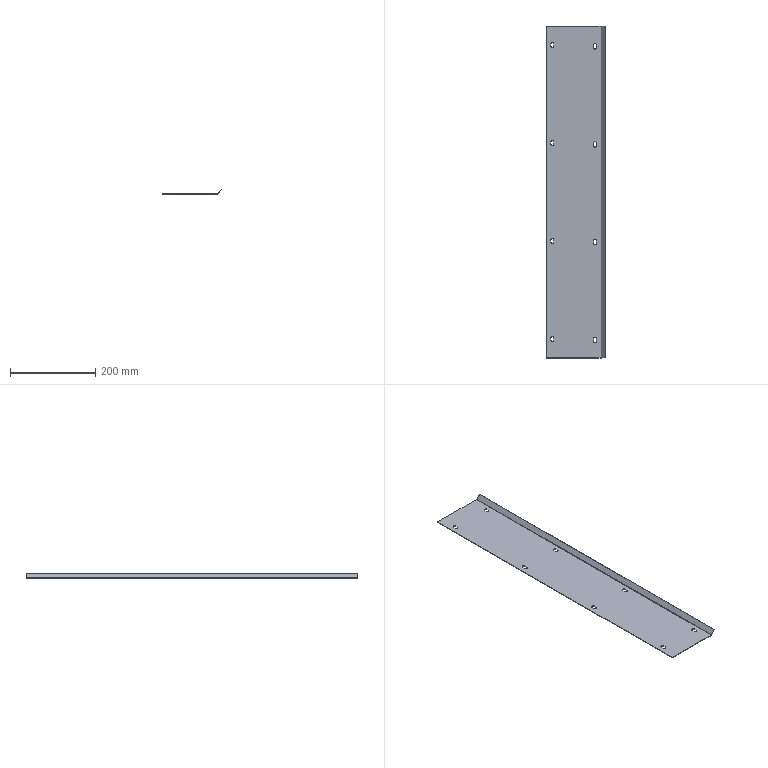Part | SolidWorks | features ICE 2, EdgeFlange 1, FlatPattern 1, LPattern 1, SMBaseFlange 1, SheetMetal 1 | 1 solid | 46 faces | box 140.607 x 780 x 11.455 mm | volume 134418 mm3 | plane 28 | cylinder 18 | commonest cylinder face diameters 7 x16 2 x1 4.4 x1
STEP:
#1=CARTESIAN_POINT('',(46.455,-345.,-1.2));
#2=VERTEX_POINT('',#1);
#3=CARTESIAN_POINT('',(46.455,-345.,0.));
#4=VERTEX_POINT('',#3);
#5=CARTESIAN_POINT('',(46.455,-345.,-10.));
#6=DIRECTION('',(0.,0.,1.));
#7=VECTOR('',#6,1000.);
#8=LINE('',#5,#7);
#9=EDGE_CURVE('',#2,#4,#8,.T.);
#10=ORIENTED_EDGE('',*,*,#9,.T.);
#11=CARTESIAN_POINT('',(46.455,-351.,0.));
#12=VERTEX_POINT('',#11);
#13=CARTESIAN_POINT('',(46.455,-345.,0.));
#14=DIRECTION('',(0.,-1.,0.));
#15=VECTOR('',#14,1000.);
#16=LINE('',#13,#15);
#17=EDGE_CURVE('',#4,#12,#16,.T.);
#18=ORIENTED_EDGE('',*,*,#17,.T.);
#19=CARTESIAN_POINT('',(46.455,-351.,-1.2));
#20=VERTEX_POINT('',#19);
#21=CARTESIAN_POINT('',(46.455,-351.,-10.));
#22=DIRECTION('',(0.,0.,1.));
#23=VECTOR('',#22,1000.);
#24=LINE('',#21,#23);
#25=EDGE_CURVE('',#20,#12,#24,.T.);
#26=ORIENTED_EDGE('',*,*,#25,.F.);
#27=CARTESIAN_POINT('',(46.455,-690.,-1.2));
#28=DIRECTION('',(0.,-1.,0.));
#29=VECTOR('',#28,1000.);
#30=LINE('',#27,#29);
#31=EDGE_CURVE('',#2,#20,#30,.T.);
#32=ORIENTED_EDGE('',*,*,#31,.F.);
#33=EDGE_LOOP('',(#10,#18,#26,#32));
#34=FACE_OUTER_BOUND('',#33,.T.);
#35=CARTESIAN_POINT('',(46.455,-345.,-10.));
#36=DIRECTION('',(-1.,0.,0.));
#37=DIRECTION('',(0.,0.,1.));
#38=AXIS2_PLACEMENT_3D('',#35,#36,#37);
#39=PLANE('',#38);
#40=ADVANCED_FACE('',(#34),#39,.F.);
#41=ORIENTED_EDGE('',*,*,#25,.T.);
#42=CARTESIAN_POINT('',(53.455,-351.,0.));
#43=VERTEX_POINT('',#42);
#44=CARTESIAN_POINT('',(49.955,-351.,0.));
#45=DIRECTION('',(0.,0.,1.));
#46=DIRECTION('',(1.,0.,0.));
#47=AXIS2_PLACEMENT_3D('',#44,#45,#46);
#48=CIRCLE('',#47,3.5);
#49=EDGE_CURVE('',#12,#43,#48,.T.);
#50=ORIENTED_EDGE('',*,*,#49,.T.);
#51=CARTESIAN_POINT('',(53.455,-351.,-1.2));
#52=VERTEX_POINT('',#51);
#53=CARTESIAN_POINT('',(53.455,-351.,-10.));
#54=DIRECTION('',(0.,0.,1.));
#55=VECTOR('',#54,1000.);
#56=LINE('',#53,#55);
#57=EDGE_CURVE('',#52,#43,#56,.T.);
#58=ORIENTED_EDGE('',*,*,#57,.F.);
#59=CARTESIAN_POINT('',(49.955,-351.,-1.2));
#60=DIRECTION('',(0.,0.,1.));
#61=DIRECTION('',(1.,0.,0.));
#62=AXIS2_PLACEMENT_3D('',#59,#60,#61);
#63=CIRCLE('',#62,3.5);
#64=EDGE_CURVE('',#20,#52,#63,.T.);
#65=ORIENTED_EDGE('',*,*,#64,.F.);
#66=EDGE_LOOP('',(#41,#50,#58,#65));
#67=FACE_OUTER_BOUND('',#66,.T.);
#68=CARTESIAN_POINT('',(49.955,-351.,-10.));
#69=DIRECTION('',(0.,0.,1.));
#70=DIRECTION('',(1.,0.,0.));
#71=AXIS2_PLACEMENT_3D('',#68,#69,#70);
#72=CYLINDRICAL_SURFACE('',#71,3.5);
#73=ADVANCED_FACE('',(#67),#72,.F.);
#74=ORIENTED_EDGE('',*,*,#57,.T.);
#75=CARTESIAN_POINT('',(53.455,-345.,0.));
#76=VERTEX_POINT('',#75);
#77=CARTESIAN_POINT('',(53.455,-345.,0.));
#78=DIRECTION('',(0.,1.,0.));
#79=VECTOR('',#78,1000.);
#80=LINE('',#77,#79);
#81=EDGE_CURVE('',#43,#76,#80,.T.);
#82=ORIENTED_EDGE('',*,*,#81,.T.);
#83=CARTESIAN_POINT('',(53.455,-345.,-1.2));
#84=VERTEX_POINT('',#83);
#85=CARTESIAN_POINT('',(53.455,-345.,-10.));
#86=DIRECTION('',(0.,0.,1.));
#87=VECTOR('',#86,1000.);
#88=LINE('',#85,#87);
#89=EDGE_CURVE('',#84,#76,#88,.T.);
#90=ORIENTED_EDGE('',*,*,#89,.F.);
#91=CARTESIAN_POINT('',(53.455,-690.,-1.2));
#92=DIRECTION('',(0.,1.,0.));
#93=VECTOR('',#92,1000.);
#94=LINE('',#91,#93);
#95=EDGE_CURVE('',#52,#84,#94,.T.);
#96=ORIENTED_EDGE('',*,*,#95,.F.);
#97=EDGE_LOOP('',(#74,#82,#90,#96));
#98=FACE_OUTER_BOUND('',#97,.T.);
#99=CARTESIAN_POINT('',(53.455,-345.,-10.));
#100=DIRECTION('',(1.,0.,0.));
#101=DIRECTION('',(0.,0.,-1.));
#102=AXIS2_PLACEMENT_3D('',#99,#100,#101);
#103=PLANE('',#102);
#104=ADVANCED_FACE('',(#98),#103,.F.);
#105=ORIENTED_EDGE('',*,*,#89,.T.);
#106=CARTESIAN_POINT('',(49.955,-345.,0.));
#107=DIRECTION('',(0.,0.,1.));
#108=DIRECTION('',(1.,0.,0.));
#109=AXIS2_PLACEMENT_3D('',#106,#107,#108);
#110=CIRCLE('',#109,3.5);
#111=EDGE_CURVE('',#76,#4,#110,.T.);
#112=ORIENTED_EDGE('',*,*,#111,.T.);
#113=ORIENTED_EDGE('',*,*,#9,.F.);
#114=CARTESIAN_POINT('',(49.955,-345.,-1.2));
#115=DIRECTION('',(0.,0.,1.));
#116=DIRECTION('',(1.,0.,0.));
#117=AXIS2_PLACEMENT_3D('',#114,#115,#116);
#118=CIRCLE('',#117,3.5);
#119=EDGE_CURVE('',#84,#2,#118,.T.);
#120=ORIENTED_EDGE('',*,*,#119,.F.);
#121=EDGE_LOOP('',(#105,#112,#113,#120));
#122=FACE_OUTER_BOUND('',#121,.T.);
#123=CARTESIAN_POINT('',(49.955,-345.,-10.));
#124=DIRECTION('',(0.,0.,1.));
#125=DIRECTION('',(1.,0.,0.));
#126=AXIS2_PLACEMENT_3D('',#123,#124,#125);
#127=CYLINDRICAL_SURFACE('',#126,3.5);
#128=ADVANCED_FACE('',(#122),#127,.F.);
#129=CARTESIAN_POINT('',(46.455,-115.,-1.2));
#130=VERTEX_POINT('',#129);
#131=CARTESIAN_POINT('',(46.455,-115.,0.));
#132=VERTEX_POINT('',#131);
#133=CARTESIAN_POINT('',(46.455,-115.,-10.));
#134=DIRECTION('',(0.,0.,1.));
#135=VECTOR('',#134,1000.);
#136=LINE('',#133,#135);
#137=EDGE_CURVE('',#130,#132,#136,.T.);
#138=ORIENTED_EDGE('',*,*,#137,.T.);
#139=CARTESIAN_POINT('',(46.455,-121.,0.));
#140=VERTEX_POINT('',#139);
#141=CARTESIAN_POINT('',(46.455,-115.,0.));
#142=DIRECTION('',(0.,-1.,0.));
#143=VECTOR('',#142,1000.);
#144=LINE('',#141,#143);
#145=EDGE_CURVE('',#132,#140,#144,.T.);
#146=ORIENTED_EDGE('',*,*,#145,.T.);
#147=CARTESIAN_POINT('',(46.455,-121.,-1.2));
#148=VERTEX_POINT('',#147);
#149=CARTESIAN_POINT('',(46.455,-121.,-10.));
#150=DIRECTION('',(0.,0.,1.));
#151=VECTOR('',#150,1000.);
#152=LINE('',#149,#151);
#153=EDGE_CURVE('',#148,#140,#152,.T.);
#154=ORIENTED_EDGE('',*,*,#153,.F.);
#155=CARTESIAN_POINT('',(46.455,-460.,-1.2));
#156=DIRECTION('',(0.,-1.,0.));
#157=VECTOR('',#156,1000.);
#158=LINE('',#155,#157);
#159=EDGE_CURVE('',#130,#148,#158,.T.);
#160=ORIENTED_EDGE('',*,*,#159,.F.);
#161=EDGE_LOOP('',(#138,#146,#154,#160));
#162=FACE_OUTER_BOUND('',#161,.T.);
#163=CARTESIAN_POINT('',(46.455,-115.,-10.));
#164=DIRECTION('',(-1.,0.,0.));
#165=DIRECTION('',(0.,0.,1.));
#166=AXIS2_PLACEMENT_3D('',#163,#164,#165);
#167=PLANE('',#166);
#168=ADVANCED_FACE('',(#162),#167,.F.);
#169=ORIENTED_EDGE('',*,*,#153,.T.);
#170=CARTESIAN_POINT('',(53.455,-121.,0.));
#171=VERTEX_POINT('',#170);
#172=CARTESIAN_POINT('',(49.955,-121.,0.));
#173=DIRECTION('',(0.,0.,1.));
#174=DIRECTION('',(1.,0.,0.));
#175=AXIS2_PLACEMENT_3D('',#172,#173,#174);
#176=CIRCLE('',#175,3.5);
#177=EDGE_CURVE('',#140,#171,#176,.T.);
#178=ORIENTED_EDGE('',*,*,#177,.T.);
#179=CARTESIAN_POINT('',(53.455,-121.,-1.2));
#180=VERTEX_POINT('',#179);
#181=CARTESIAN_POINT('',(53.455,-121.,-10.));
#182=DIRECTION('',(0.,0.,1.));
#183=VECTOR('',#182,1000.);
#184=LINE('',#181,#183);
#185=EDGE_CURVE('',#180,#171,#184,.T.);
#186=ORIENTED_EDGE('',*,*,#185,.F.);
#187=CARTESIAN_POINT('',(49.955,-121.,-1.2));
#188=DIRECTION('',(0.,0.,1.));
#189=DIRECTION('',(1.,0.,0.));
#190=AXIS2_PLACEMENT_3D('',#187,#188,#189);
#191=CIRCLE('',#190,3.5);
#192=EDGE_CURVE('',#148,#180,#191,.T.);
#193=ORIENTED_EDGE('',*,*,#192,.F.);
#194=EDGE_LOOP('',(#169,#178,#186,#193));
#195=FACE_OUTER_BOUND('',#194,.T.);
#196=CARTESIAN_POINT('',(49.955,-121.,-10.));
#197=DIRECTION('',(0.,0.,1.));
#198=DIRECTION('',(1.,0.,0.));
#199=AXIS2_PLACEMENT_3D('',#196,#197,#198);
#200=CYLINDRICAL_SURFACE('',#199,3.5);
#201=ADVANCED_FACE('',(#195),#200,.F.);
#202=ORIENTED_EDGE('',*,*,#185,.T.);
#203=CARTESIAN_POINT('',(53.455,-115.,0.));
#204=VERTEX_POINT('',#203);
#205=CARTESIAN_POINT('',(53.455,-115.,0.));
#206=DIRECTION('',(0.,1.,0.));
#207=VECTOR('',#206,1000.);
#208=LINE('',#205,#207);
#209=EDGE_CURVE('',#171,#204,#208,.T.);
#210=ORIENTED_EDGE('',*,*,#209,.T.);
#211=CARTESIAN_POINT('',(53.455,-115.,-1.2));
#212=VERTEX_POINT('',#211);
#213=CARTESIAN_POINT('',(53.455,-115.,-10.));
#214=DIRECTION('',(0.,0.,1.));
#215=VECTOR('',#214,1000.);
#216=LINE('',#213,#215);
#217=EDGE_CURVE('',#212,#204,#216,.T.);
#218=ORIENTED_EDGE('',*,*,#217,.F.);
#219=CARTESIAN_POINT('',(53.455,-460.,-1.2));
#220=DIRECTION('',(0.,1.,0.));
#221=VECTOR('',#220,1000.);
#222=LINE('',#219,#221);
#223=EDGE_CURVE('',#180,#212,#222,.T.);
#224=ORIENTED_EDGE('',*,*,#223,.F.);
#225=EDGE_LOOP('',(#202,#210,#218,#224));
#226=FACE_OUTER_BOUND('',#225,.T.);
#227=CARTESIAN_POINT('',(53.455,-115.,-10.));
#228=DIRECTION('',(1.,0.,0.));
#229=DIRECTION('',(0.,0.,-1.));
#230=AXIS2_PLACEMENT_3D('',#227,#228,#229);
#231=PLANE('',#230);
#232=ADVANCED_FACE('',(#226),#231,.F.);
#233=ORIENTED_EDGE('',*,*,#217,.T.);
#234=CARTESIAN_POINT('',(49.955,-115.,0.));
#235=DIRECTION('',(0.,0.,1.));
#236=DIRECTION('',(1.,0.,0.));
#237=AXIS2_PLACEMENT_3D('',#234,#235,#236);
#238=CIRCLE('',#237,3.5);
#239=EDGE_CURVE('',#204,#132,#238,.T.);
#240=ORIENTED_EDGE('',*,*,#239,.T.);
#241=ORIENTED_EDGE('',*,*,#137,.F.);
#242=CARTESIAN_POINT('',(49.955,-115.,-1.2));
#243=DIRECTION('',(0.,0.,1.));
#244=DIRECTION('',(1.,0.,0.));
#245=AXIS2_PLACEMENT_3D('',#242,#243,#244);
#246=CIRCLE('',#245,3.5);
#247=EDGE_CURVE('',#212,#130,#246,.T.);
#248=ORIENTED_EDGE('',*,*,#247,.F.);
#249=EDGE_LOOP('',(#233,#240,#241,#248));
#250=FACE_OUTER_BOUND('',#249,.T.);
#251=CARTESIAN_POINT('',(49.955,-115.,-10.));
#252=DIRECTION('',(0.,0.,1.));
#253=DIRECTION('',(1.,0.,0.));
#254=AXIS2_PLACEMENT_3D('',#251,#252,#253);
#255=CYLINDRICAL_SURFACE('',#254,3.5);
#256=ADVANCED_FACE('',(#250),#255,.F.);
#257=CARTESIAN_POINT('',(-53.5,-342.,-1.2));
#258=VERTEX_POINT('',#257);
#259=CARTESIAN_POINT('',(-53.5,-342.,0.));
#260=VERTEX_POINT('',#259);
#261=CARTESIAN_POINT('',(-53.5,-342.,-10.));
#262=DIRECTION('',(0.,0.,1.));
#263=VECTOR('',#262,1000.);
#264=LINE('',#261,#263);
#265=EDGE_CURVE('',#258,#260,#264,.T.);
#266=ORIENTED_EDGE('',*,*,#265,.T.);
#267=CARTESIAN_POINT('',(-53.5,-348.,0.));
#268=VERTEX_POINT('',#267);
#269=CARTESIAN_POINT('',(-53.5,-342.,0.));
#270=DIRECTION('',(0.,-1.,0.));
#271=VECTOR('',#270,1000.);
#272=LINE('',#269,#271);
#273=EDGE_CURVE('',#260,#268,#272,.T.);
#274=ORIENTED_EDGE('',*,*,#273,.T.);
#275=CARTESIAN_POINT('',(-53.5,-348.,-1.2));
#276=VERTEX_POINT('',#275);
#277=CARTESIAN_POINT('',(-53.5,-348.,-10.));
#278=DIRECTION('',(0.,0.,1.));
#279=VECTOR('',#278,1000.);
#280=LINE('',#277,#279);
#281=EDGE_CURVE('',#276,#268,#280,.T.);
#282=ORIENTED_EDGE('',*,*,#281,.F.);
#283=CARTESIAN_POINT('',(-53.5,-690.,-1.2));
#284=DIRECTION('',(0.,-1.,0.));
#285=VECTOR('',#284,1000.);
#286=LINE('',#283,#285);
#287=EDGE_CURVE('',#258,#276,#286,.T.);
#288=ORIENTED_EDGE('',*,*,#287,.F.);
#289=EDGE_LOOP('',(#266,#274,#282,#288));
#290=FACE_OUTER_BOUND('',#289,.T.);
#291=CARTESIAN_POINT('',(-53.5,-342.,-10.));
#292=DIRECTION('',(-1.,0.,0.));
#293=DIRECTION('',(0.,-1.,0.));
#294=AXIS2_PLACEMENT_3D('',#291,#292,#293);
#295=PLANE('',#294);
#296=ADVANCED_FACE('',(#290),#295,.F.);
#297=ORIENTED_EDGE('',*,*,#281,.T.);
#298=CARTESIAN_POINT('',(-46.5,-348.,0.));
#299=VERTEX_POINT('',#298);
#300=CARTESIAN_POINT('',(-50.,-348.,0.));
#301=DIRECTION('',(0.,0.,1.));
#302=DIRECTION('',(1.,0.,0.));
#303=AXIS2_PLACEMENT_3D('',#300,#301,#302);
#304=CIRCLE('',#303,3.5);
#305=EDGE_CURVE('',#268,#299,#304,.T.);
#306=ORIENTED_EDGE('',*,*,#305,.T.);
#307=CARTESIAN_POINT('',(-46.5,-348.,-1.2));
#308=VERTEX_POINT('',#307);
#309=CARTESIAN_POINT('',(-46.5,-348.,-10.));
#310=DIRECTION('',(0.,0.,1.));
#311=VECTOR('',#310,1000.);
#312=LINE('',#309,#311);
#313=EDGE_CURVE('',#308,#299,#312,.T.);
#314=ORIENTED_EDGE('',*,*,#313,.F.);
#315=CARTESIAN_POINT('',(-50.,-348.,-1.2));
#316=DIRECTION('',(0.,0.,1.));
#317=DIRECTION('',(1.,0.,0.));
#318=AXIS2_PLACEMENT_3D('',#315,#316,#317);
#319=CIRCLE('',#318,3.5);
#320=EDGE_CURVE('',#276,#308,#319,.T.);
#321=ORIENTED_EDGE('',*,*,#320,.F.);
#322=EDGE_LOOP('',(#297,#306,#314,#321));
#323=FACE_OUTER_BOUND('',#322,.T.);
#324=CARTESIAN_POINT('',(-50.,-348.,-10.));
#325=DIRECTION('',(0.,0.,1.));
#326=DIRECTION('',(1.,0.,0.));
#327=AXIS2_PLACEMENT_3D('',#324,#325,#326);
#328=CYLINDRICAL_SURFACE('',#327,3.5);
#329=ADVANCED_FACE('',(#323),#328,.F.);
#330=ORIENTED_EDGE('',*,*,#313,.T.);
#331=CARTESIAN_POINT('',(-46.5,-342.,0.));
#332=VERTEX_POINT('',#331);
#333=CARTESIAN_POINT('',(-46.5,-342.,0.));
#334=DIRECTION('',(0.,1.,0.));
#335=VECTOR('',#334,1000.);
#336=LINE('',#333,#335);
#337=EDGE_CURVE('',#299,#332,#336,.T.);
#338=ORIENTED_EDGE('',*,*,#337,.T.);
#339=CARTESIAN_POINT('',(-46.5,-342.,-1.2));
#340=VERTEX_POINT('',#339);
#341=CARTESIAN_POINT('',(-46.5,-342.,-10.));
#342=DIRECTION('',(0.,0.,1.));
#343=VECTOR('',#342,1000.);
#344=LINE('',#341,#343);
#345=EDGE_CURVE('',#340,#332,#344,.T.);
#346=ORIENTED_EDGE('',*,*,#345,.F.);
#347=CARTESIAN_POINT('',(-46.5,-690.,-1.2));
#348=DIRECTION('',(0.,1.,0.));
#349=VECTOR('',#348,1000.);
#350=LINE('',#347,#349);
#351=EDGE_CURVE('',#308,#340,#350,.T.);
#352=ORIENTED_EDGE('',*,*,#351,.F.);
#353=EDGE_LOOP('',(#330,#338,#346,#352));
#354=FACE_OUTER_BOUND('',#353,.T.);
#355=CARTESIAN_POINT('',(-46.5,-342.,-10.));
#356=DIRECTION('',(1.,0.,0.));
#357=DIRECTION('',(0.,1.,0.));
#358=AXIS2_PLACEMENT_3D('',#355,#356,#357);
#359=PLANE('',#358);
#360=ADVANCED_FACE('',(#354),#359,.F.);
#361=ORIENTED_EDGE('',*,*,#345,.T.);
#362=CARTESIAN_POINT('',(-50.,-342.,0.));
#363=DIRECTION('',(0.,0.,1.));
#364=DIRECTION('',(1.,0.,0.));
#365=AXIS2_PLACEMENT_3D('',#362,#363,#364);
#366=CIRCLE('',#365,3.5);
#367=EDGE_CURVE('',#332,#260,#366,.T.);
#368=ORIENTED_EDGE('',*,*,#367,.T.);
#369=ORIENTED_EDGE('',*,*,#265,.F.);
#370=CARTESIAN_POINT('',(-50.,-342.,-1.2));
#371=DIRECTION('',(0.,0.,1.));
#372=DIRECTION('',(1.,0.,0.));
#373=AXIS2_PLACEMENT_3D('',#370,#371,#372);
#374=CIRCLE('',#373,3.5);
#375=EDGE_CURVE('',#340,#258,#374,.T.);
#376=ORIENTED_EDGE('',*,*,#375,.F.);
#377=EDGE_LOOP('',(#361,#368,#369,#376));
#378=FACE_OUTER_BOUND('',#377,.T.);
#379=CARTESIAN_POINT('',(-50.,-342.,-10.));
#380=DIRECTION('',(0.,0.,1.));
#381=DIRECTION('',(1.,0.,0.));
#382=AXIS2_PLACEMENT_3D('',#379,#380,#381);
#383=CYLINDRICAL_SURFACE('',#382,3.5);
#384=ADVANCED_FACE('',(#378),#383,.F.);
#385=CARTESIAN_POINT('',(-53.5,-112.,-1.2));
#386=VERTEX_POINT('',#385);
#387=CARTESIAN_POINT('',(-53.5,-112.,0.));
#388=VERTEX_POINT('',#387);
#389=CARTESIAN_POINT('',(-53.5,-112.,-10.));
#390=DIRECTION('',(0.,0.,1.));
#391=VECTOR('',#390,1000.);
#392=LINE('',#389,#391);
#393=EDGE_CURVE('',#386,#388,#392,.T.);
#394=ORIENTED_EDGE('',*,*,#393,.T.);
#395=CARTESIAN_POINT('',(-53.5,-118.,0.));
#396=VERTEX_POINT('',#395);
#397=CARTESIAN_POINT('',(-53.5,-112.,0.));
#398=DIRECTION('',(0.,-1.,0.));
#399=VECTOR('',#398,1000.);
#400=LINE('',#397,#399);
#401=EDGE_CURVE('',#388,#396,#400,.T.);
#402=ORIENTED_EDGE('',*,*,#401,.T.);
#403=CARTESIAN_POINT('',(-53.5,-118.,-1.2));
#404=VERTEX_POINT('',#403);
#405=CARTESIAN_POINT('',(-53.5,-118.,-10.));
#406=DIRECTION('',(0.,0.,1.));
#407=VECTOR('',#406,1000.);
#408=LINE('',#405,#407);
#409=EDGE_CURVE('',#404,#396,#408,.T.);
#410=ORIENTED_EDGE('',*,*,#409,.F.);
#411=CARTESIAN_POINT('',(-53.5,-460.,-1.2));
#412=DIRECTION('',(0.,-1.,0.));
#413=VECTOR('',#412,1000.);
#414=LINE('',#411,#413);
#415=EDGE_CURVE('',#386,#404,#414,.T.);
#416=ORIENTED_EDGE('',*,*,#415,.F.);
#417=EDGE_LOOP('',(#394,#402,#410,#416));
#418=FACE_OUTER_BOUND('',#417,.T.);
#419=CARTESIAN_POINT('',(-53.5,-112.,-10.));
#420=DIRECTION('',(-1.,0.,0.));
#421=DIRECTION('',(0.,-1.,0.));
#422=AXIS2_PLACEMENT_3D('',#419,#420,#421);
#423=PLANE('',#422);
#424=ADVANCED_FACE('',(#418),#423,.F.);
#425=ORIENTED_EDGE('',*,*,#409,.T.);
#426=CARTESIAN_POINT('',(-46.5,-118.,0.));
#427=VERTEX_POINT('',#426);
#428=CARTESIAN_POINT('',(-50.,-118.,0.));
#429=DIRECTION('',(0.,0.,1.));
#430=DIRECTION('',(1.,0.,0.));
#431=AXIS2_PLACEMENT_3D('',#428,#429,#430);
#432=CIRCLE('',#431,3.5);
#433=EDGE_CURVE('',#396,#427,#432,.T.);
#434=ORIENTED_EDGE('',*,*,#433,.T.);
#435=CARTESIAN_POINT('',(-46.5,-118.,-1.2));
#436=VERTEX_POINT('',#435);
#437=CARTESIAN_POINT('',(-46.5,-118.,-10.));
#438=DIRECTION('',(0.,0.,1.));
#439=VECTOR('',#438,1000.);
#440=LINE('',#437,#439);
#441=EDGE_CURVE('',#436,#427,#440,.T.);
#442=ORIENTED_EDGE('',*,*,#441,.F.);
#443=CARTESIAN_POINT('',(-50.,-118.,-1.2));
#444=DIRECTION('',(0.,0.,1.));
#445=DIRECTION('',(1.,0.,0.));
#446=AXIS2_PLACEMENT_3D('',#443,#444,#445);
#447=CIRCLE('',#446,3.5);
#448=EDGE_CURVE('',#404,#436,#447,.T.);
#449=ORIENTED_EDGE('',*,*,#448,.F.);
#450=EDGE_LOOP('',(#425,#434,#442,#449));
#451=FACE_OUTER_BOUND('',#450,.T.);
#452=CARTESIAN_POINT('',(-50.,-118.,-10.));
#453=DIRECTION('',(0.,0.,1.));
#454=DIRECTION('',(1.,0.,0.));
#455=AXIS2_PLACEMENT_3D('',#452,#453,#454);
#456=CYLINDRICAL_SURFACE('',#455,3.5);
#457=ADVANCED_FACE('',(#451),#456,.F.);
#458=ORIENTED_EDGE('',*,*,#441,.T.);
#459=CARTESIAN_POINT('',(-46.5,-112.,0.));
#460=VERTEX_POINT('',#459);
#461=CARTESIAN_POINT('',(-46.5,-112.,0.));
#462=DIRECTION('',(0.,1.,0.));
#463=VECTOR('',#462,1000.);
#464=LINE('',#461,#463);
#465=EDGE_CURVE('',#427,#460,#464,.T.);
#466=ORIENTED_EDGE('',*,*,#465,.T.);
#467=CARTESIAN_POINT('',(-46.5,-112.,-1.2));
#468=VERTEX_POINT('',#467);
#469=CARTESIAN_POINT('',(-46.5,-112.,-10.));
#470=DIRECTION('',(0.,0.,1.));
#471=VECTOR('',#470,1000.);
#472=LINE('',#469,#471);
#473=EDGE_CURVE('',#468,#460,#472,.T.);
#474=ORIENTED_EDGE('',*,*,#473,.F.);
#475=CARTESIAN_POINT('',(-46.5,-460.,-1.2));
#476=DIRECTION('',(0.,1.,0.));
#477=VECTOR('',#476,1000.);
#478=LINE('',#475,#477);
#479=EDGE_CURVE('',#436,#468,#478,.T.);
#480=ORIENTED_EDGE('',*,*,#479,.F.);
#481=EDGE_LOOP('',(#458,#466,#474,#480));
#482=FACE_OUTER_BOUND('',#481,.T.);
#483=CARTESIAN_POINT('',(-46.5,-112.,-10.));
#484=DIRECTION('',(1.,0.,0.));
#485=DIRECTION('',(0.,1.,0.));
#486=AXIS2_PLACEMENT_3D('',#483,#484,#485);
#487=PLANE('',#486);
#488=ADVANCED_FACE('',(#482),#487,.F.);
#489=ORIENTED_EDGE('',*,*,#473,.T.);
#490=CARTESIAN_POINT('',(-50.,-112.,0.));
#491=DIRECTION('',(0.,0.,1.));
#492=DIRECTION('',(1.,0.,0.));
#493=AXIS2_PLACEMENT_3D('',#490,#491,#492);
#494=CIRCLE('',#493,3.5);
#495=EDGE_CURVE('',#460,#388,#494,.T.);
#496=ORIENTED_EDGE('',*,*,#495,.T.);
#497=ORIENTED_EDGE('',*,*,#393,.F.);
#498=CARTESIAN_POINT('',(-50.,-112.,-1.2));
#499=DIRECTION('',(0.,0.,1.));
#500=DIRECTION('',(1.,0.,0.));
#501=AXIS2_PLACEMENT_3D('',#498,#499,#500);
#502=CIRCLE('',#501,3.5);
#503=EDGE_CURVE('',#468,#386,#502,.T.);
#504=ORIENTED_EDGE('',*,*,#503,.F.);
#505=EDGE_LOOP('',(#489,#496,#497,#504));
#506=FACE_OUTER_BOUND('',#505,.T.);
#507=CARTESIAN_POINT('',(-50.,-112.,-10.));
#508=DIRECTION('',(0.,0.,1.));
#509=DIRECTION('',(1.,0.,0.));
#510=AXIS2_PLACEMENT_3D('',#507,#508,#509);
#511=CYLINDRICAL_SURFACE('',#510,3.5);
#512=ADVANCED_FACE('',(#506),#511,.F.);
#513=CARTESIAN_POINT('',(64.089,390.,0.));
#514=VERTEX_POINT('',#513);
#515=CARTESIAN_POINT('',(-65.,390.,0.));
#516=VERTEX_POINT('',#515);
#517=CARTESIAN_POINT('',(-65.,390.,0.));
#518=DIRECTION('',(-1.,0.,0.));
#519=VECTOR('',#518,1000.);
#520=LINE('',#517,#519);
#521=EDGE_CURVE('',#514,#516,#520,.T.);
#522=ORIENTED_EDGE('',*,*,#521,.F.);
#523=CARTESIAN_POINT('',(64.089,390.,-1.2));
#524=VERTEX_POINT('',#523);
#525=CARTESIAN_POINT('',(64.089,390.,0.));
#526=DIRECTION('',(0.,0.,-1.));
#527=VECTOR('',#526,1000.);
#528=LINE('',#525,#527);
#529=EDGE_CURVE('',#514,#524,#528,.T.);
#530=ORIENTED_EDGE('',*,*,#529,.T.);
#531=CARTESIAN_POINT('',(-65.,390.,-1.2));
#532=VERTEX_POINT('',#531);
#533=CARTESIAN_POINT('',(-65.,390.,-1.2));
#534=DIRECTION('',(-1.,0.,0.));
#535=VECTOR('',#534,1000.);
#536=LINE('',#533,#535);
#537=EDGE_CURVE('',#524,#532,#536,.T.);
#538=ORIENTED_EDGE('',*,*,#537,.T.);
#539=CARTESIAN_POINT('',(-65.,390.,-1.2));
#540=DIRECTION('',(0.,0.,1.));
#541=VECTOR('',#540,1000.);
#542=LINE('',#539,#541);
#543=EDGE_CURVE('',#532,#516,#542,.T.);
#544=ORIENTED_EDGE('',*,*,#543,.T.);
#545=EDGE_LOOP('',(#522,#530,#538,#544));
#546=FACE_OUTER_BOUND('',#545,.T.);
#547=CARTESIAN_POINT('',(-65.,390.,-1.2));
#548=DIRECTION('',(0.,1.,0.));
#549=DIRECTION('',(0.,0.,1.));
#550=AXIS2_PLACEMENT_3D('',#547,#548,#549);
#551=PLANE('',#550);
#552=ADVANCED_FACE('',(#546),#551,.T.);
#553=CARTESIAN_POINT('',(53.455,109.,-1.2));
#554=VERTEX_POINT('',#553);
#555=CARTESIAN_POINT('',(53.455,115.,-1.2));
#556=VERTEX_POINT('',#555);
#557=CARTESIAN_POINT('',(53.455,-230.,-1.2));
#558=DIRECTION('',(0.,1.,0.));
#559=VECTOR('',#558,1000.);
#560=LINE('',#557,#559);
#561=EDGE_CURVE('',#554,#556,#560,.T.);
#562=ORIENTED_EDGE('',*,*,#561,.T.);
#563=CARTESIAN_POINT('',(46.455,115.,-1.2));
#564=VERTEX_POINT('',#563);
#565=CARTESIAN_POINT('',(49.955,115.,-1.2));
#566=DIRECTION('',(0.,0.,1.));
#567=DIRECTION('',(1.,0.,0.));
#568=AXIS2_PLACEMENT_3D('',#565,#566,#567);
#569=CIRCLE('',#568,3.5);
#570=EDGE_CURVE('',#556,#564,#569,.T.);
#571=ORIENTED_EDGE('',*,*,#570,.T.);
#572=CARTESIAN_POINT('',(46.455,109.,-1.2));
#573=VERTEX_POINT('',#572);
#574=CARTESIAN_POINT('',(46.455,-230.,-1.2));
#575=DIRECTION('',(0.,-1.,0.));
#576=VECTOR('',#575,1000.);
#577=LINE('',#574,#576);
#578=EDGE_CURVE('',#564,#573,#577,.T.);
#579=ORIENTED_EDGE('',*,*,#578,.T.);
#580=CARTESIAN_POINT('',(49.955,109.,-1.2));
#581=DIRECTION('',(0.,0.,1.));
#582=DIRECTION('',(1.,0.,0.));
#583=AXIS2_PLACEMENT_3D('',#580,#581,#582);
#584=CIRCLE('',#583,3.5);
#585=EDGE_CURVE('',#573,#554,#584,.T.);
#586=ORIENTED_EDGE('',*,*,#585,.T.);
#587=EDGE_LOOP('',(#562,#571,#579,#586));
#588=FACE_BOUND('',#587,.T.);
#589=CARTESIAN_POINT('',(-46.5,112.,-1.2));
#590=VERTEX_POINT('',#589);
#591=CARTESIAN_POINT('',(-46.5,118.,-1.2));
#592=VERTEX_POINT('',#591);
#593=CARTESIAN_POINT('',(-46.5,-230.,-1.2));
#594=DIRECTION('',(0.,1.,0.));
#595=VECTOR('',#594,1000.);
#596=LINE('',#593,#595);
#597=EDGE_CURVE('',#590,#592,#596,.T.);
#598=ORIENTED_EDGE('',*,*,#597,.T.);
#599=CARTESIAN_POINT('',(-53.5,118.,-1.2));
#600=VERTEX_POINT('',#599);
#601=CARTESIAN_POINT('',(-50.,118.,-1.2));
#602=DIRECTION('',(0.,0.,1.));
#603=DIRECTION('',(1.,0.,0.));
#604=AXIS2_PLACEMENT_3D('',#601,#602,#603);
#605=CIRCLE('',#604,3.5);
#606=EDGE_CURVE('',#592,#600,#605,.T.);
#607=ORIENTED_EDGE('',*,*,#606,.T.);
#608=CARTESIAN_POINT('',(-53.5,112.,-1.2));
#609=VERTEX_POINT('',#608);
#610=CARTESIAN_POINT('',(-53.5,-230.,-1.2));
#611=DIRECTION('',(0.,-1.,0.));
#612=VECTOR('',#611,1000.);
#613=LINE('',#610,#612);
#614=EDGE_CURVE('',#600,#609,#613,.T.);
#615=ORIENTED_EDGE('',*,*,#614,.T.);
#616=CARTESIAN_POINT('',(-50.,112.,-1.2));
#617=DIRECTION('',(0.,0.,1.));
#618=DIRECTION('',(1.,0.,0.));
#619=AXIS2_PLACEMENT_3D('',#616,#617,#618);
#620=CIRCLE('',#619,3.5);
#621=EDGE_CURVE('',#609,#590,#620,.T.);
#622=ORIENTED_EDGE('',*,*,#621,.T.);
#623=EDGE_LOOP('',(#598,#607,#615,#622));
#624=FACE_BOUND('',#623,.T.);
#625=CARTESIAN_POINT('',(-46.5,342.,-1.2));
#626=VERTEX_POINT('',#625);
#627=CARTESIAN_POINT('',(-46.5,348.,-1.2));
#628=VERTEX_POINT('',#627);
#629=CARTESIAN_POINT('',(-46.5,0.,-1.2));
#630=DIRECTION('',(0.,1.,0.));
#631=VECTOR('',#630,1000.);
#632=LINE('',#629,#631);
#633=EDGE_CURVE('',#626,#628,#632,.T.);
#634=ORIENTED_EDGE('',*,*,#633,.T.);
#635=CARTESIAN_POINT('',(-53.5,348.,-1.2));
#636=VERTEX_POINT('',#635);
#637=CARTESIAN_POINT('',(-50.,348.,-1.2));
#638=DIRECTION('',(0.,0.,1.));
#639=DIRECTION('',(1.,0.,0.));
#640=AXIS2_PLACEMENT_3D('',#637,#638,#639);
#641=CIRCLE('',#640,3.5);
#642=EDGE_CURVE('',#628,#636,#641,.T.);
#643=ORIENTED_EDGE('',*,*,#642,.T.);
#644=CARTESIAN_POINT('',(-53.5,342.,-1.2));
#645=VERTEX_POINT('',#644);
#646=CARTESIAN_POINT('',(-53.5,0.,-1.2));
#647=DIRECTION('',(0.,-1.,0.));
#648=VECTOR('',#647,1000.);
#649=LINE('',#646,#648);
#650=EDGE_CURVE('',#636,#645,#649,.T.);
#651=ORIENTED_EDGE('',*,*,#650,.T.);
#652=CARTESIAN_POINT('',(-50.,342.,-1.2));
#653=DIRECTION('',(0.,0.,1.));
#654=DIRECTION('',(1.,0.,0.));
#655=AXIS2_PLACEMENT_3D('',#652,#653,#654);
#656=CIRCLE('',#655,3.5);
#657=EDGE_CURVE('',#645,#626,#656,.T.);
#658=ORIENTED_EDGE('',*,*,#657,.T.);
#659=EDGE_LOOP('',(#634,#643,#651,#658));
#660=FACE_BOUND('',#659,.T.);
#661=CARTESIAN_POINT('',(53.455,339.,-1.2));
#662=VERTEX_POINT('',#661);
#663=CARTESIAN_POINT('',(53.455,345.,-1.2));
#664=VERTEX_POINT('',#663);
#665=CARTESIAN_POINT('',(53.455,0.,-1.2));
#666=DIRECTION('',(0.,1.,0.));
#667=VECTOR('',#666,1000.);
#668=LINE('',#665,#667);
#669=EDGE_CURVE('',#662,#664,#668,.T.);
#670=ORIENTED_EDGE('',*,*,#669,.T.);
#671=CARTESIAN_POINT('',(46.455,345.,-1.2));
#672=VERTEX_POINT('',#671);
#673=CARTESIAN_POINT('',(49.955,345.,-1.2));
#674=DIRECTION('',(0.,0.,1.));
#675=DIRECTION('',(1.,0.,0.));
#676=AXIS2_PLACEMENT_3D('',#673,#674,#675);
#677=CIRCLE('',#676,3.5);
#678=EDGE_CURVE('',#664,#672,#677,.T.);
#679=ORIENTED_EDGE('',*,*,#678,.T.);
#680=CARTESIAN_POINT('',(46.455,339.,-1.2));
#681=VERTEX_POINT('',#680);
#682=CARTESIAN_POINT('',(46.455,0.,-1.2));
#683=DIRECTION('',(0.,-1.,0.));
#684=VECTOR('',#683,1000.);
#685=LINE('',#682,#684);
#686=EDGE_CURVE('',#672,#681,#685,.T.);
#687=ORIENTED_EDGE('',*,*,#686,.T.);
#688=CARTESIAN_POINT('',(49.955,339.,-1.2));
#689=DIRECTION('',(0.,0.,1.));
#690=DIRECTION('',(1.,0.,0.));
#691=AXIS2_PLACEMENT_3D('',#688,#689,#690);
#692=CIRCLE('',#691,3.5);
#693=EDGE_CURVE('',#681,#662,#692,.T.);
#694=ORIENTED_EDGE('',*,*,#693,.T.);
#695=EDGE_LOOP('',(#670,#679,#687,#694));
#696=FACE_BOUND('',#695,.T.);
#697=CARTESIAN_POINT('',(64.089,-390.,-1.2));
#698=VERTEX_POINT('',#697);
#699=CARTESIAN_POINT('',(64.089,390.,-1.2));
#700=DIRECTION('',(0.,-1.,0.));
#701=VECTOR('',#700,1000.);
#702=LINE('',#699,#701);
#703=EDGE_CURVE('',#524,#698,#702,.T.);
#704=ORIENTED_EDGE('',*,*,#703,.T.);
#705=CARTESIAN_POINT('',(-65.,-390.,-1.2));
#706=VERTEX_POINT('',#705);
#707=CARTESIAN_POINT('',(-65.,-390.,-1.2));
#708=DIRECTION('',(1.,0.,0.));
#709=VECTOR('',#708,1000.);
#710=LINE('',#707,#709);
#711=EDGE_CURVE('',#706,#698,#710,.T.);
#712=ORIENTED_EDGE('',*,*,#711,.F.);
#713=CARTESIAN_POINT('',(-65.,390.,-1.2));
#714=DIRECTION('',(0.,-1.,0.));
#715=VECTOR('',#714,1000.);
#716=LINE('',#713,#715);
#717=EDGE_CURVE('',#532,#706,#716,.T.);
#718=ORIENTED_EDGE('',*,*,#717,.F.);
#719=ORIENTED_EDGE('',*,*,#537,.F.);
#720=EDGE_LOOP('',(#704,#712,#718,#719));
#721=FACE_OUTER_BOUND('',#720,.T.);
#722=ORIENTED_EDGE('',*,*,#503,.T.);
#723=ORIENTED_EDGE('',*,*,#415,.T.);
#724=ORIENTED_EDGE('',*,*,#448,.T.);
#725=ORIENTED_EDGE('',*,*,#479,.T.);
#726=EDGE_LOOP('',(#722,#723,#724,#725));
#727=FACE_BOUND('',#726,.T.);
#728=ORIENTED_EDGE('',*,*,#375,.T.);
#729=ORIENTED_EDGE('',*,*,#287,.T.);
#730=ORIENTED_EDGE('',*,*,#320,.T.);
#731=ORIENTED_EDGE('',*,*,#351,.T.);
#732=EDGE_LOOP('',(#728,#729,#730,#731));
#733=FACE_BOUND('',#732,.T.);
#734=ORIENTED_EDGE('',*,*,#247,.T.);
#735=ORIENTED_EDGE('',*,*,#159,.T.);
#736=ORIENTED_EDGE('',*,*,#192,.T.);
#737=ORIENTED_EDGE('',*,*,#223,.T.);
#738=EDGE_LOOP('',(#734,#735,#736,#737));
#739=FACE_BOUND('',#738,.T.);
#740=ORIENTED_EDGE('',*,*,#119,.T.);
#741=ORIENTED_EDGE('',*,*,#31,.T.);
#742=ORIENTED_EDGE('',*,*,#64,.T.);
#743=ORIENTED_EDGE('',*,*,#95,.T.);
#744=EDGE_LOOP('',(#740,#741,#742,#743));
#745=FACE_BOUND('',#744,.T.);
#746=CARTESIAN_POINT('',(0.,0.,-1.2));
#747=DIRECTION('',(0.,0.,1.));
#748=DIRECTION('',(1.,0.,0.));
#749=AXIS2_PLACEMENT_3D('',#746,#747,#748);
#750=PLANE('',#749);
#751=ADVANCED_FACE('',(#588,#624,#660,#696,#721,#727,#733,#739,#745),#750,.F.);
#752=CARTESIAN_POINT('',(53.455,115.,0.));
#753=VERTEX_POINT('',#752);
#754=CARTESIAN_POINT('',(46.455,115.,0.));
#755=VERTEX_POINT('',#754);
#756=CARTESIAN_POINT('',(49.955,115.,0.));
#757=DIRECTION('',(0.,0.,1.));
#758=DIRECTION('',(1.,0.,0.));
#759=AXIS2_PLACEMENT_3D('',#756,#757,#758);
#760=CIRCLE('',#759,3.5);
#761=EDGE_CURVE('',#753,#755,#760,.T.);
#762=ORIENTED_EDGE('',*,*,#761,.F.);
#763=CARTESIAN_POINT('',(53.455,109.,0.));
#764=VERTEX_POINT('',#763);
#765=CARTESIAN_POINT('',(53.455,115.,0.));
#766=DIRECTION('',(0.,1.,0.));
#767=VECTOR('',#766,1000.);
#768=LINE('',#765,#767);
#769=EDGE_CURVE('',#764,#753,#768,.T.);
#770=ORIENTED_EDGE('',*,*,#769,.F.);
#771=CARTESIAN_POINT('',(46.455,109.,0.));
#772=VERTEX_POINT('',#771);
#773=CARTESIAN_POINT('',(49.955,109.,0.));
#774=DIRECTION('',(0.,0.,1.));
#775=DIRECTION('',(1.,0.,0.));
#776=AXIS2_PLACEMENT_3D('',#773,#774,#775);
#777=CIRCLE('',#776,3.5);
#778=EDGE_CURVE('',#772,#764,#777,.T.);
#779=ORIENTED_EDGE('',*,*,#778,.F.);
#780=CARTESIAN_POINT('',(46.455,115.,0.));
#781=DIRECTION('',(0.,-1.,0.));
#782=VECTOR('',#781,1000.);
#783=LINE('',#780,#782);
#784=EDGE_CURVE('',#755,#772,#783,.T.);
#785=ORIENTED_EDGE('',*,*,#784,.F.);
#786=EDGE_LOOP('',(#762,#770,#779,#785));
#787=FACE_BOUND('',#786,.T.);
#788=CARTESIAN_POINT('',(-46.5,118.,0.));
#789=VERTEX_POINT('',#788);
#790=CARTESIAN_POINT('',(-53.5,118.,0.));
#791=VERTEX_POINT('',#790);
#792=CARTESIAN_POINT('',(-50.,118.,0.));
#793=DIRECTION('',(0.,0.,1.));
#794=DIRECTION('',(1.,0.,0.));
#795=AXIS2_PLACEMENT_3D('',#792,#793,#794);
#796=CIRCLE('',#795,3.5);
#797=EDGE_CURVE('',#789,#791,#796,.T.);
#798=ORIENTED_EDGE('',*,*,#797,.F.);
#799=CARTESIAN_POINT('',(-46.5,112.,0.));
#800=VERTEX_POINT('',#799);
#801=CARTESIAN_POINT('',(-46.5,118.,0.));
#802=DIRECTION('',(0.,1.,0.));
#803=VECTOR('',#802,1000.);
#804=LINE('',#801,#803);
#805=EDGE_CURVE('',#800,#789,#804,.T.);
#806=ORIENTED_EDGE('',*,*,#805,.F.);
#807=CARTESIAN_POINT('',(-53.5,112.,0.));
#808=VERTEX_POINT('',#807);
#809=CARTESIAN_POINT('',(-50.,112.,0.));
#810=DIRECTION('',(0.,0.,1.));
#811=DIRECTION('',(1.,0.,0.));
#812=AXIS2_PLACEMENT_3D('',#809,#810,#811);
#813=CIRCLE('',#812,3.5);
#814=EDGE_CURVE('',#808,#800,#813,.T.);
#815=ORIENTED_EDGE('',*,*,#814,.F.);
#816=CARTESIAN_POINT('',(-53.5,118.,0.));
#817=DIRECTION('',(0.,-1.,0.));
#818=VECTOR('',#817,1000.);
#819=LINE('',#816,#818);
#820=EDGE_CURVE('',#791,#808,#819,.T.);
#821=ORIENTED_EDGE('',*,*,#820,.F.);
#822=EDGE_LOOP('',(#798,#806,#815,#821));
#823=FACE_BOUND('',#822,.T.);
#824=CARTESIAN_POINT('',(-46.5,348.,0.));
#825=VERTEX_POINT('',#824);
#826=CARTESIAN_POINT('',(-53.5,348.,0.));
#827=VERTEX_POINT('',#826);
#828=CARTESIAN_POINT('',(-50.,348.,0.));
#829=DIRECTION('',(0.,0.,1.));
#830=DIRECTION('',(1.,0.,0.));
#831=AXIS2_PLACEMENT_3D('',#828,#829,#830);
#832=CIRCLE('',#831,3.5);
#833=EDGE_CURVE('',#825,#827,#832,.T.);
#834=ORIENTED_EDGE('',*,*,#833,.F.);
#835=CARTESIAN_POINT('',(-46.5,342.,0.));
#836=VERTEX_POINT('',#835);
#837=CARTESIAN_POINT('',(-46.5,348.,0.));
#838=DIRECTION('',(0.,1.,0.));
#839=VECTOR('',#838,1000.);
#840=LINE('',#837,#839);
#841=EDGE_CURVE('',#836,#825,#840,.T.);
#842=ORIENTED_EDGE('',*,*,#841,.F.);
#843=CARTESIAN_POINT('',(-53.5,342.,0.));
#844=VERTEX_POINT('',#843);
#845=CARTESIAN_POINT('',(-50.,342.,0.));
#846=DIRECTION('',(0.,0.,1.));
#847=DIRECTION('',(1.,0.,0.));
#848=AXIS2_PLACEMENT_3D('',#845,#846,#847);
#849=CIRCLE('',#848,3.5);
#850=EDGE_CURVE('',#844,#836,#849,.T.);
#851=ORIENTED_EDGE('',*,*,#850,.F.);
#852=CARTESIAN_POINT('',(-53.5,348.,0.));
#853=DIRECTION('',(0.,-1.,0.));
#854=VECTOR('',#853,1000.);
#855=LINE('',#852,#854);
#856=EDGE_CURVE('',#827,#844,#855,.T.);
#857=ORIENTED_EDGE('',*,*,#856,.F.);
#858=EDGE_LOOP('',(#834,#842,#851,#857));
#859=FACE_BOUND('',#858,.T.);
#860=CARTESIAN_POINT('',(53.455,345.,0.));
#861=VERTEX_POINT('',#860);
#862=CARTESIAN_POINT('',(46.455,345.,0.));
#863=VERTEX_POINT('',#862);
#864=CARTESIAN_POINT('',(49.955,345.,0.));
#865=DIRECTION('',(0.,0.,1.));
#866=DIRECTION('',(1.,0.,0.));
#867=AXIS2_PLACEMENT_3D('',#864,#865,#866);
#868=CIRCLE('',#867,3.5);
#869=EDGE_CURVE('',#861,#863,#868,.T.);
#870=ORIENTED_EDGE('',*,*,#869,.F.);
#871=CARTESIAN_POINT('',(53.455,339.,0.));
#872=VERTEX_POINT('',#871);
#873=CARTESIAN_POINT('',(53.455,345.,0.));
#874=DIRECTION('',(0.,1.,0.));
#875=VECTOR('',#874,1000.);
#876=LINE('',#873,#875);
#877=EDGE_CURVE('',#872,#861,#876,.T.);
#878=ORIENTED_EDGE('',*,*,#877,.F.);
#879=CARTESIAN_POINT('',(46.455,339.,0.));
#880=VERTEX_POINT('',#879);
#881=CARTESIAN_POINT('',(49.955,339.,0.));
#882=DIRECTION('',(0.,0.,1.));
#883=DIRECTION('',(1.,0.,0.));
#884=AXIS2_PLACEMENT_3D('',#881,#882,#883);
#885=CIRCLE('',#884,3.5);
#886=EDGE_CURVE('',#880,#872,#885,.T.);
#887=ORIENTED_EDGE('',*,*,#886,.F.);
#888=CARTESIAN_POINT('',(46.455,345.,0.));
#889=DIRECTION('',(0.,-1.,0.));
#890=VECTOR('',#889,1000.);
#891=LINE('',#888,#890);
#892=EDGE_CURVE('',#863,#880,#891,.T.);
#893=ORIENTED_EDGE('',*,*,#892,.F.);
#894=EDGE_LOOP('',(#870,#878,#887,#893));
#895=FACE_BOUND('',#894,.T.);
#896=CARTESIAN_POINT('',(-65.,-390.,0.));
#897=VERTEX_POINT('',#896);
#898=CARTESIAN_POINT('',(64.089,-390.,0.));
#899=VERTEX_POINT('',#898);
#900=CARTESIAN_POINT('',(-65.,-390.,0.));
#901=DIRECTION('',(1.,0.,0.));
#902=VECTOR('',#901,1000.);
#903=LINE('',#900,#902);
#904=EDGE_CURVE('',#897,#899,#903,.T.);
#905=ORIENTED_EDGE('',*,*,#904,.T.);
#906=CARTESIAN_POINT('',(64.089,390.,0.));
#907=DIRECTION('',(0.,-1.,0.));
#908=VECTOR('',#907,1000.);
#909=LINE('',#906,#908);
#910=EDGE_CURVE('',#514,#899,#909,.T.);
#911=ORIENTED_EDGE('',*,*,#910,.F.);
#912=ORIENTED_EDGE('',*,*,#521,.T.);
#913=CARTESIAN_POINT('',(-65.,390.,0.));
#914=DIRECTION('',(0.,-1.,0.));
#915=VECTOR('',#914,1000.);
#916=LINE('',#913,#915);
#917=EDGE_CURVE('',#516,#897,#916,.T.);
#918=ORIENTED_EDGE('',*,*,#917,.T.);
#919=EDGE_LOOP('',(#905,#911,#912,#918));
#920=FACE_OUTER_BOUND('',#919,.T.);
#921=ORIENTED_EDGE('',*,*,#495,.F.);
#922=ORIENTED_EDGE('',*,*,#465,.F.);
#923=ORIENTED_EDGE('',*,*,#433,.F.);
#924=ORIENTED_EDGE('',*,*,#401,.F.);
#925=EDGE_LOOP('',(#921,#922,#923,#924));
#926=FACE_BOUND('',#925,.T.);
#927=ORIENTED_EDGE('',*,*,#367,.F.);
#928=ORIENTED_EDGE('',*,*,#337,.F.);
#929=ORIENTED_EDGE('',*,*,#305,.F.);
#930=ORIENTED_EDGE('',*,*,#273,.F.);
#931=EDGE_LOOP('',(#927,#928,#929,#930));
#932=FACE_BOUND('',#931,.T.);
#933=ORIENTED_EDGE('',*,*,#239,.F.);
#934=ORIENTED_EDGE('',*,*,#209,.F.);
#935=ORIENTED_EDGE('',*,*,#177,.F.);
#936=ORIENTED_EDGE('',*,*,#145,.F.);
#937=EDGE_LOOP('',(#933,#934,#935,#936));
#938=FACE_BOUND('',#937,.T.);
#939=ORIENTED_EDGE('',*,*,#111,.F.);
#940=ORIENTED_EDGE('',*,*,#81,.F.);
#941=ORIENTED_EDGE('',*,*,#49,.F.);
#942=ORIENTED_EDGE('',*,*,#17,.F.);
#943=EDGE_LOOP('',(#939,#940,#941,#942));
#944=FACE_BOUND('',#943,.T.);
#945=CARTESIAN_POINT('',(0.,0.,0.));
#946=DIRECTION('',(0.,0.,1.));
#947=DIRECTION('',(1.,0.,0.));
#948=AXIS2_PLACEMENT_3D('',#945,#946,#947);
#949=PLANE('',#948);
#950=ADVANCED_FACE('',(#787,#823,#859,#895,#920,#926,#932,#938,#944),#949,.T.);
#951=CARTESIAN_POINT('',(64.089,-390.,0.));
#952=DIRECTION('',(0.,0.,-1.));
#953=VECTOR('',#952,1000.);
#954=LINE('',#951,#953);
#955=EDGE_CURVE('',#899,#698,#954,.T.);
#956=ORIENTED_EDGE('',*,*,#955,.F.);
#957=ORIENTED_EDGE('',*,*,#904,.F.);
#958=CARTESIAN_POINT('',(-65.,-390.,-1.2));
#959=DIRECTION('',(0.,0.,1.));
#960=VECTOR('',#959,1000.);
#961=LINE('',#958,#960);
#962=EDGE_CURVE('',#706,#897,#961,.T.);
#963=ORIENTED_EDGE('',*,*,#962,.F.);
#964=ORIENTED_EDGE('',*,*,#711,.T.);
#965=EDGE_LOOP('',(#956,#957,#963,#964));
#966=FACE_OUTER_BOUND('',#965,.T.);
#967=CARTESIAN_POINT('',(-65.,-390.,-1.2));
#968=DIRECTION('',(0.,-1.,0.));
#969=DIRECTION('',(0.,0.,-1.));
#970=AXIS2_PLACEMENT_3D('',#967,#968,#969);
#971=PLANE('',#970);
#972=ADVANCED_FACE('',(#966),#971,.T.);
#973=ORIENTED_EDGE('',*,*,#917,.F.);
#974=ORIENTED_EDGE('',*,*,#543,.F.);
#975=ORIENTED_EDGE('',*,*,#717,.T.);
#976=ORIENTED_EDGE('',*,*,#962,.T.);
#977=EDGE_LOOP('',(#973,#974,#975,#976));
#978=FACE_OUTER_BOUND('',#977,.T.);
#979=CARTESIAN_POINT('',(-65.,390.,-1.2));
#980=DIRECTION('',(-1.,0.,0.));
#981=DIRECTION('',(0.,-1.,0.));
#982=AXIS2_PLACEMENT_3D('',#979,#980,#981);
#983=PLANE('',#982);
#984=ADVANCED_FACE('',(#978),#983,.T.);
#985=CARTESIAN_POINT('',(64.796,-390.,0.2929));
#986=VERTEX_POINT('',#985);
#987=CARTESIAN_POINT('',(65.644,-390.,-0.5556));
#988=VERTEX_POINT('',#987);
#989=CARTESIAN_POINT('',(65.644,-390.,-0.5556));
#990=DIRECTION('',(0.7071,0.,-0.7071));
#991=VECTOR('',#990,1000.);
#992=LINE('',#989,#991);
#993=EDGE_CURVE('',#986,#988,#992,.T.);
#994=ORIENTED_EDGE('',*,*,#993,.F.);
#995=CARTESIAN_POINT('',(64.089,-390.,1.));
#996=DIRECTION('',(0.,-1.,0.));
#997=DIRECTION('',(0.,0.,1.));
#998=AXIS2_PLACEMENT_3D('',#995,#996,#997);
#999=CIRCLE('',#998,1.);
#1000=EDGE_CURVE('',#899,#986,#999,.T.);
#1001=ORIENTED_EDGE('',*,*,#1000,.F.);
#1002=ORIENTED_EDGE('',*,*,#955,.T.);
#1003=CARTESIAN_POINT('',(64.089,-390.,1.));
#1004=DIRECTION('',(0.,-1.,0.));
#1005=DIRECTION('',(0.,0.,1.));
#1006=AXIS2_PLACEMENT_3D('',#1003,#1004,#1005);
#1007=CIRCLE('',#1006,2.2);
#1008=EDGE_CURVE('',#698,#988,#1007,.T.);
#1009=ORIENTED_EDGE('',*,*,#1008,.T.);
#1010=EDGE_LOOP('',(#994,#1001,#1002,#1009));
#1011=FACE_OUTER_BOUND('',#1010,.T.);
#1012=CARTESIAN_POINT('',(64.089,-390.,1.));
#1013=DIRECTION('',(0.,-1.,0.));
#1014=DIRECTION('',(0.,0.,-1.));
#1015=AXIS2_PLACEMENT_3D('',#1012,#1013,#1014);
#1016=PLANE('',#1015);
#1017=ADVANCED_FACE('',(#1011),#1016,.T.);
#1018=CARTESIAN_POINT('',(64.796,390.,0.2929));
#1019=VERTEX_POINT('',#1018);
#1020=CARTESIAN_POINT('',(64.089,390.,1.));
#1021=DIRECTION('',(0.,1.,0.));
#1022=DIRECTION('',(0.,0.,1.));
#1023=AXIS2_PLACEMENT_3D('',#1020,#1021,#1022);
#1024=CIRCLE('',#1023,1.);
#1025=EDGE_CURVE('',#1019,#514,#1024,.T.);
#1026=ORIENTED_EDGE('',*,*,#1025,.F.);
#1027=CARTESIAN_POINT('',(65.644,390.,-0.5556));
#1028=VERTEX_POINT('',#1027);
#1029=CARTESIAN_POINT('',(64.796,390.,0.2929));
#1030=DIRECTION('',(0.7071,0.,-0.7071));
#1031=VECTOR('',#1030,1000.);
#1032=LINE('',#1029,#1031);
#1033=EDGE_CURVE('',#1019,#1028,#1032,.T.);
#1034=ORIENTED_EDGE('',*,*,#1033,.T.);
#1035=CARTESIAN_POINT('',(64.089,390.,1.));
#1036=DIRECTION('',(0.,1.,0.));
#1037=DIRECTION('',(0.,0.,1.));
#1038=AXIS2_PLACEMENT_3D('',#1035,#1036,#1037);
#1039=CIRCLE('',#1038,2.2);
#1040=EDGE_CURVE('',#1028,#524,#1039,.T.);
#1041=ORIENTED_EDGE('',*,*,#1040,.T.);
#1042=ORIENTED_EDGE('',*,*,#529,.F.);
#1043=EDGE_LOOP('',(#1026,#1034,#1041,#1042));
#1044=FACE_OUTER_BOUND('',#1043,.T.);
#1045=CARTESIAN_POINT('',(64.089,390.,1.));
#1046=DIRECTION('',(0.,-1.,0.));
#1047=DIRECTION('',(0.,0.,-1.));
#1048=AXIS2_PLACEMENT_3D('',#1045,#1046,#1047);
#1049=PLANE('',#1048);
#1050=ADVANCED_FACE('',(#1044),#1049,.F.);
#1051=ORIENTED_EDGE('',*,*,#703,.F.);
#1052=ORIENTED_EDGE('',*,*,#1040,.F.);
#1053=CARTESIAN_POINT('',(65.644,-390.,-0.5556));
#1054=DIRECTION('',(0.,-1.,0.));
#1055=VECTOR('',#1054,1000.);
#1056=LINE('',#1053,#1055);
#1057=EDGE_CURVE('',#1028,#988,#1056,.T.);
#1058=ORIENTED_EDGE('',*,*,#1057,.T.);
#1059=ORIENTED_EDGE('',*,*,#1008,.F.);
#1060=EDGE_LOOP('',(#1051,#1052,#1058,#1059));
#1061=FACE_OUTER_BOUND('',#1060,.T.);
#1062=CARTESIAN_POINT('',(64.089,390.,1.));
#1063=DIRECTION('',(0.,1.,0.));
#1064=DIRECTION('',(0.7071,0.,-0.7071));
#1065=AXIS2_PLACEMENT_3D('',#1062,#1063,#1064);
#1066=CYLINDRICAL_SURFACE('',#1065,2.2);
#1067=ADVANCED_FACE('',(#1061),#1066,.T.);
#1068=ORIENTED_EDGE('',*,*,#910,.T.);
#1069=ORIENTED_EDGE('',*,*,#1000,.T.);
#1070=CARTESIAN_POINT('',(64.796,-390.,0.2929));
#1071=DIRECTION('',(0.,1.,0.));
#1072=VECTOR('',#1071,1000.);
#1073=LINE('',#1070,#1072);
#1074=EDGE_CURVE('',#986,#1019,#1073,.T.);
#1075=ORIENTED_EDGE('',*,*,#1074,.T.);
#1076=ORIENTED_EDGE('',*,*,#1025,.T.);
#1077=EDGE_LOOP('',(#1068,#1069,#1075,#1076));
#1078=FACE_OUTER_BOUND('',#1077,.T.);
#1079=CARTESIAN_POINT('',(64.089,390.,1.));
#1080=DIRECTION('',(0.,1.,0.));
#1081=DIRECTION('',(0.7071,0.,-0.7071));
#1082=AXIS2_PLACEMENT_3D('',#1079,#1080,#1081);
#1083=CYLINDRICAL_SURFACE('',#1082,1.);
#1084=ADVANCED_FACE('',(#1078),#1083,.F.);
#1085=ORIENTED_EDGE('',*,*,#1033,.F.);
#1086=CARTESIAN_POINT('',(74.758,390.,10.255));
#1087=VERTEX_POINT('',#1086);
#1088=CARTESIAN_POINT('',(74.758,390.,10.255));
#1089=DIRECTION('',(0.7071,0.,0.7071));
#1090=VECTOR('',#1089,1000.);
#1091=LINE('',#1088,#1090);
#1092=EDGE_CURVE('',#1019,#1087,#1091,.T.);
#1093=ORIENTED_EDGE('',*,*,#1092,.T.);
#1094=CARTESIAN_POINT('',(75.607,390.,9.407));
#1095=VERTEX_POINT('',#1094);
#1096=CARTESIAN_POINT('',(75.607,390.,9.407));
#1097=DIRECTION('',(-0.7071,0.,0.7071));
#1098=VECTOR('',#1097,1000.);
#1099=LINE('',#1096,#1098);
#1100=EDGE_CURVE('',#1095,#1087,#1099,.T.);
#1101=ORIENTED_EDGE('',*,*,#1100,.F.);
#1102=CARTESIAN_POINT('',(32.851,390.,-33.349));
#1103=DIRECTION('',(0.7071,0.,0.7071));
#1104=VECTOR('',#1103,1000.);
#1105=LINE('',#1102,#1104);
#1106=EDGE_CURVE('',#1028,#1095,#1105,.T.);
#1107=ORIENTED_EDGE('',*,*,#1106,.F.);
#1108=EDGE_LOOP('',(#1085,#1093,#1101,#1107));
#1109=FACE_OUTER_BOUND('',#1108,.T.);
#1110=CARTESIAN_POINT('',(75.607,390.,9.407));
#1111=DIRECTION('',(0.,-1.,0.));
#1112=DIRECTION('',(1.,0.,0.));
#1113=AXIS2_PLACEMENT_3D('',#1110,#1111,#1112);
#1114=PLANE('',#1113);
#1115=ADVANCED_FACE('',(#1109),#1114,.F.);
#1116=ORIENTED_EDGE('',*,*,#993,.T.);
#1117=CARTESIAN_POINT('',(75.607,-390.,9.407));
#1118=VERTEX_POINT('',#1117);
#1119=CARTESIAN_POINT('',(32.851,-390.,-33.349));
#1120=DIRECTION('',(-0.7071,0.,-0.7071));
#1121=VECTOR('',#1120,1000.);
#1122=LINE('',#1119,#1121);
#1123=EDGE_CURVE('',#1118,#988,#1122,.T.);
#1124=ORIENTED_EDGE('',*,*,#1123,.F.);
#1125=CARTESIAN_POINT('',(74.758,-390.,10.255));
#1126=VERTEX_POINT('',#1125);
#1127=CARTESIAN_POINT('',(75.607,-390.,9.407));
#1128=DIRECTION('',(-0.7071,0.,0.7071));
#1129=VECTOR('',#1128,1000.);
#1130=LINE('',#1127,#1129);
#1131=EDGE_CURVE('',#1118,#1126,#1130,.T.);
#1132=ORIENTED_EDGE('',*,*,#1131,.T.);
#1133=CARTESIAN_POINT('',(64.503,-390.,0.));
#1134=DIRECTION('',(-0.7071,0.,-0.7071));
#1135=VECTOR('',#1134,1000.);
#1136=LINE('',#1133,#1135);
#1137=EDGE_CURVE('',#1126,#986,#1136,.T.);
#1138=ORIENTED_EDGE('',*,*,#1137,.T.);
#1139=EDGE_LOOP('',(#1116,#1124,#1132,#1138));
#1140=FACE_OUTER_BOUND('',#1139,.T.);
#1141=CARTESIAN_POINT('',(65.351,-390.,-0.8485));
#1142=DIRECTION('',(0.,1.,0.));
#1143=DIRECTION('',(0.,0.,1.));
#1144=AXIS2_PLACEMENT_3D('',#1141,#1142,#1143);
#1145=PLANE('',#1144);
#1146=ADVANCED_FACE('',(#1140),#1145,.F.);
#1147=ORIENTED_EDGE('',*,*,#1057,.F.);
#1148=ORIENTED_EDGE('',*,*,#1106,.T.);
#1149=CARTESIAN_POINT('',(75.607,0.,9.407));
#1150=DIRECTION('',(0.,-1.,0.));
#1151=VECTOR('',#1150,1000.);
#1152=LINE('',#1149,#1151);
#1153=EDGE_CURVE('',#1095,#1118,#1152,.T.);
#1154=ORIENTED_EDGE('',*,*,#1153,.T.);
#1155=ORIENTED_EDGE('',*,*,#1123,.T.);
#1156=EDGE_LOOP('',(#1147,#1148,#1154,#1155));
#1157=FACE_OUTER_BOUND('',#1156,.T.);
#1158=CARTESIAN_POINT('',(32.851,0.,-33.349));
#1159=DIRECTION('',(-0.7071,0.,0.7071));
#1160=DIRECTION('',(0.7071,0.,0.7071));
#1161=AXIS2_PLACEMENT_3D('',#1158,#1159,#1160);
#1162=PLANE('',#1161);
#1163=ADVANCED_FACE('',(#1157),#1162,.F.);
#1164=ORIENTED_EDGE('',*,*,#1092,.F.);
#1165=ORIENTED_EDGE('',*,*,#1074,.F.);
#1166=ORIENTED_EDGE('',*,*,#1137,.F.);
#1167=CARTESIAN_POINT('',(74.758,-390.,10.255));
#1168=DIRECTION('',(0.,-1.,0.));
#1169=VECTOR('',#1168,1000.);
#1170=LINE('',#1167,#1169);
#1171=EDGE_CURVE('',#1087,#1126,#1170,.T.);
#1172=ORIENTED_EDGE('',*,*,#1171,.F.);
#1173=EDGE_LOOP('',(#1164,#1165,#1166,#1172));
#1174=FACE_OUTER_BOUND('',#1173,.T.);
#1175=CARTESIAN_POINT('',(32.003,0.,-32.5));
#1176=DIRECTION('',(-0.7071,0.,0.7071));
#1177=DIRECTION('',(0.7071,0.,0.7071));
#1178=AXIS2_PLACEMENT_3D('',#1175,#1176,#1177);
#1179=PLANE('',#1178);
#1180=ADVANCED_FACE('',(#1174),#1179,.T.);
#1181=ORIENTED_EDGE('',*,*,#1171,.T.);
#1182=ORIENTED_EDGE('',*,*,#1131,.F.);
#1183=ORIENTED_EDGE('',*,*,#1153,.F.);
#1184=ORIENTED_EDGE('',*,*,#1100,.T.);
#1185=EDGE_LOOP('',(#1181,#1182,#1183,#1184));
#1186=FACE_OUTER_BOUND('',#1185,.T.);
#1187=CARTESIAN_POINT('',(75.607,-390.,9.407));
#1188=DIRECTION('',(-0.7071,0.,-0.7071));
#1189=DIRECTION('',(-0.7071,0.,0.7071));
#1190=AXIS2_PLACEMENT_3D('',#1187,#1188,#1189);
#1191=PLANE('',#1190);
#1192=ADVANCED_FACE('',(#1186),#1191,.F.);
#1193=CARTESIAN_POINT('',(53.455,345.,-10.));
#1194=DIRECTION('',(0.,0.,1.));
#1195=VECTOR('',#1194,1000.);
#1196=LINE('',#1193,#1195);
#1197=EDGE_CURVE('',#664,#861,#1196,.T.);
#1198=ORIENTED_EDGE('',*,*,#1197,.T.);
#1199=ORIENTED_EDGE('',*,*,#869,.T.);
#1200=CARTESIAN_POINT('',(46.455,345.,-10.));
#1201=DIRECTION('',(0.,0.,1.));
#1202=VECTOR('',#1201,1000.);
#1203=LINE('',#1200,#1202);
#1204=EDGE_CURVE('',#672,#863,#1203,.T.);
#1205=ORIENTED_EDGE('',*,*,#1204,.F.);
#1206=ORIENTED_EDGE('',*,*,#678,.F.);
#1207=EDGE_LOOP('',(#1198,#1199,#1205,#1206));
#1208=FACE_OUTER_BOUND('',#1207,.T.);
#1209=CARTESIAN_POINT('',(49.955,345.,-10.));
#1210=DIRECTION('',(0.,0.,1.));
#1211=DIRECTION('',(1.,0.,0.));
#1212=AXIS2_PLACEMENT_3D('',#1209,#1210,#1211);
#1213=CYLINDRICAL_SURFACE('',#1212,3.5);
#1214=ADVANCED_FACE('',(#1208),#1213,.F.);
#1215=CARTESIAN_POINT('',(53.455,339.,-10.));
#1216=DIRECTION('',(0.,0.,1.));
#1217=VECTOR('',#1216,1000.);
#1218=LINE('',#1215,#1217);
#1219=EDGE_CURVE('',#662,#872,#1218,.T.);
#1220=ORIENTED_EDGE('',*,*,#1219,.T.);
#1221=ORIENTED_EDGE('',*,*,#877,.T.);
#1222=ORIENTED_EDGE('',*,*,#1197,.F.);
#1223=ORIENTED_EDGE('',*,*,#669,.F.);
#1224=EDGE_LOOP('',(#1220,#1221,#1222,#1223));
#1225=FACE_OUTER_BOUND('',#1224,.T.);
#1226=CARTESIAN_POINT('',(53.455,345.,-10.));
#1227=DIRECTION('',(1.,0.,0.));
#1228=DIRECTION('',(0.,0.,-1.));
#1229=AXIS2_PLACEMENT_3D('',#1226,#1227,#1228);
#1230=PLANE('',#1229);
#1231=ADVANCED_FACE('',(#1225),#1230,.F.);
#1232=CARTESIAN_POINT('',(46.455,339.,-10.));
#1233=DIRECTION('',(0.,0.,1.));
#1234=VECTOR('',#1233,1000.);
#1235=LINE('',#1232,#1234);
#1236=EDGE_CURVE('',#681,#880,#1235,.T.);
#1237=ORIENTED_EDGE('',*,*,#1236,.T.);
#1238=ORIENTED_EDGE('',*,*,#886,.T.);
#1239=ORIENTED_EDGE('',*,*,#1219,.F.);
#1240=ORIENTED_EDGE('',*,*,#693,.F.);
#1241=EDGE_LOOP('',(#1237,#1238,#1239,#1240));
#1242=FACE_OUTER_BOUND('',#1241,.T.);
#1243=CARTESIAN_POINT('',(49.955,339.,-10.));
#1244=DIRECTION('',(0.,0.,1.));
#1245=DIRECTION('',(1.,0.,0.));
#1246=AXIS2_PLACEMENT_3D('',#1243,#1244,#1245);
#1247=CYLINDRICAL_SURFACE('',#1246,3.5);
#1248=ADVANCED_FACE('',(#1242),#1247,.F.);
#1249=ORIENTED_EDGE('',*,*,#1204,.T.);
#1250=ORIENTED_EDGE('',*,*,#892,.T.);
#1251=ORIENTED_EDGE('',*,*,#1236,.F.);
#1252=ORIENTED_EDGE('',*,*,#686,.F.);
#1253=EDGE_LOOP('',(#1249,#1250,#1251,#1252));
#1254=FACE_OUTER_BOUND('',#1253,.T.);
#1255=CARTESIAN_POINT('',(46.455,345.,-10.));
#1256=DIRECTION('',(-1.,0.,0.));
#1257=DIRECTION('',(0.,0.,1.));
#1258=AXIS2_PLACEMENT_3D('',#1255,#1256,#1257);
#1259=PLANE('',#1258);
#1260=ADVANCED_FACE('',(#1254),#1259,.F.);
#1261=CARTESIAN_POINT('',(-46.5,348.,-10.));
#1262=DIRECTION('',(0.,0.,1.));
#1263=VECTOR('',#1262,1000.);
#1264=LINE('',#1261,#1263);
#1265=EDGE_CURVE('',#628,#825,#1264,.T.);
#1266=ORIENTED_EDGE('',*,*,#1265,.T.);
#1267=ORIENTED_EDGE('',*,*,#833,.T.);
#1268=CARTESIAN_POINT('',(-53.5,348.,-10.));
#1269=DIRECTION('',(0.,0.,1.));
#1270=VECTOR('',#1269,1000.);
#1271=LINE('',#1268,#1270);
#1272=EDGE_CURVE('',#636,#827,#1271,.T.);
#1273=ORIENTED_EDGE('',*,*,#1272,.F.);
#1274=ORIENTED_EDGE('',*,*,#642,.F.);
#1275=EDGE_LOOP('',(#1266,#1267,#1273,#1274));
#1276=FACE_OUTER_BOUND('',#1275,.T.);
#1277=CARTESIAN_POINT('',(-50.,348.,-10.));
#1278=DIRECTION('',(0.,0.,1.));
#1279=DIRECTION('',(1.,0.,0.));
#1280=AXIS2_PLACEMENT_3D('',#1277,#1278,#1279);
#1281=CYLINDRICAL_SURFACE('',#1280,3.5);
#1282=ADVANCED_FACE('',(#1276),#1281,.F.);
#1283=CARTESIAN_POINT('',(-46.5,342.,-10.));
#1284=DIRECTION('',(0.,0.,1.));
#1285=VECTOR('',#1284,1000.);
#1286=LINE('',#1283,#1285);
#1287=EDGE_CURVE('',#626,#836,#1286,.T.);
#1288=ORIENTED_EDGE('',*,*,#1287,.T.);
#1289=ORIENTED_EDGE('',*,*,#841,.T.);
#1290=ORIENTED_EDGE('',*,*,#1265,.F.);
#1291=ORIENTED_EDGE('',*,*,#633,.F.);
#1292=EDGE_LOOP('',(#1288,#1289,#1290,#1291));
#1293=FACE_OUTER_BOUND('',#1292,.T.);
#1294=CARTESIAN_POINT('',(-46.5,348.,-10.));
#1295=DIRECTION('',(1.,0.,0.));
#1296=DIRECTION('',(0.,1.,0.));
#1297=AXIS2_PLACEMENT_3D('',#1294,#1295,#1296);
#1298=PLANE('',#1297);
#1299=ADVANCED_FACE('',(#1293),#1298,.F.);
#1300=CARTESIAN_POINT('',(-53.5,342.,-10.));
#1301=DIRECTION('',(0.,0.,1.));
#1302=VECTOR('',#1301,1000.);
#1303=LINE('',#1300,#1302);
#1304=EDGE_CURVE('',#645,#844,#1303,.T.);
#1305=ORIENTED_EDGE('',*,*,#1304,.T.);
#1306=ORIENTED_EDGE('',*,*,#850,.T.);
#1307=ORIENTED_EDGE('',*,*,#1287,.F.);
#1308=ORIENTED_EDGE('',*,*,#657,.F.);
#1309=EDGE_LOOP('',(#1305,#1306,#1307,#1308));
#1310=FACE_OUTER_BOUND('',#1309,.T.);
#1311=CARTESIAN_POINT('',(-50.,342.,-10.));
#1312=DIRECTION('',(0.,0.,1.));
#1313=DIRECTION('',(1.,0.,0.));
#1314=AXIS2_PLACEMENT_3D('',#1311,#1312,#1313);
#1315=CYLINDRICAL_SURFACE('',#1314,3.5);
#1316=ADVANCED_FACE('',(#1310),#1315,.F.);
#1317=ORIENTED_EDGE('',*,*,#1272,.T.);
#1318=ORIENTED_EDGE('',*,*,#856,.T.);
#1319=ORIENTED_EDGE('',*,*,#1304,.F.);
#1320=ORIENTED_EDGE('',*,*,#650,.F.);
#1321=EDGE_LOOP('',(#1317,#1318,#1319,#1320));
#1322=FACE_OUTER_BOUND('',#1321,.T.);
#1323=CARTESIAN_POINT('',(-53.5,348.,-10.));
#1324=DIRECTION('',(-1.,0.,0.));
#1325=DIRECTION('',(0.,-1.,0.));
#1326=AXIS2_PLACEMENT_3D('',#1323,#1324,#1325);
#1327=PLANE('',#1326);
#1328=ADVANCED_FACE('',(#1322),#1327,.F.);
#1329=CARTESIAN_POINT('',(-46.5,118.,-10.));
#1330=DIRECTION('',(0.,0.,1.));
#1331=VECTOR('',#1330,1000.);
#1332=LINE('',#1329,#1331);
#1333=EDGE_CURVE('',#592,#789,#1332,.T.);
#1334=ORIENTED_EDGE('',*,*,#1333,.T.);
#1335=ORIENTED_EDGE('',*,*,#797,.T.);
#1336=CARTESIAN_POINT('',(-53.5,118.,-10.));
#1337=DIRECTION('',(0.,0.,1.));
#1338=VECTOR('',#1337,1000.);
#1339=LINE('',#1336,#1338);
#1340=EDGE_CURVE('',#600,#791,#1339,.T.);
#1341=ORIENTED_EDGE('',*,*,#1340,.F.);
#1342=ORIENTED_EDGE('',*,*,#606,.F.);
#1343=EDGE_LOOP('',(#1334,#1335,#1341,#1342));
#1344=FACE_OUTER_BOUND('',#1343,.T.);
#1345=CARTESIAN_POINT('',(-50.,118.,-10.));
#1346=DIRECTION('',(0.,0.,1.));
#1347=DIRECTION('',(1.,0.,0.));
#1348=AXIS2_PLACEMENT_3D('',#1345,#1346,#1347);
#1349=CYLINDRICAL_SURFACE('',#1348,3.5);
#1350=ADVANCED_FACE('',(#1344),#1349,.F.);
#1351=CARTESIAN_POINT('',(-46.5,112.,-10.));
#1352=DIRECTION('',(0.,0.,1.));
#1353=VECTOR('',#1352,1000.);
#1354=LINE('',#1351,#1353);
#1355=EDGE_CURVE('',#590,#800,#1354,.T.);
#1356=ORIENTED_EDGE('',*,*,#1355,.T.);
#1357=ORIENTED_EDGE('',*,*,#805,.T.);
#1358=ORIENTED_EDGE('',*,*,#1333,.F.);
#1359=ORIENTED_EDGE('',*,*,#597,.F.);
#1360=EDGE_LOOP('',(#1356,#1357,#1358,#1359));
#1361=FACE_OUTER_BOUND('',#1360,.T.);
#1362=CARTESIAN_POINT('',(-46.5,118.,-10.));
#1363=DIRECTION('',(1.,0.,0.));
#1364=DIRECTION('',(0.,1.,0.));
#1365=AXIS2_PLACEMENT_3D('',#1362,#1363,#1364);
#1366=PLANE('',#1365);
#1367=ADVANCED_FACE('',(#1361),#1366,.F.);
#1368=CARTESIAN_POINT('',(-53.5,112.,-10.));
#1369=DIRECTION('',(0.,0.,1.));
#1370=VECTOR('',#1369,1000.);
#1371=LINE('',#1368,#1370);
#1372=EDGE_CURVE('',#609,#808,#1371,.T.);
#1373=ORIENTED_EDGE('',*,*,#1372,.T.);
#1374=ORIENTED_EDGE('',*,*,#814,.T.);
#1375=ORIENTED_EDGE('',*,*,#1355,.F.);
#1376=ORIENTED_EDGE('',*,*,#621,.F.);
#1377=EDGE_LOOP('',(#1373,#1374,#1375,#1376));
#1378=FACE_OUTER_BOUND('',#1377,.T.);
#1379=CARTESIAN_POINT('',(-50.,112.,-10.));
#1380=DIRECTION('',(0.,0.,1.));
#1381=DIRECTION('',(1.,0.,0.));
#1382=AXIS2_PLACEMENT_3D('',#1379,#1380,#1381);
#1383=CYLINDRICAL_SURFACE('',#1382,3.5);
#1384=ADVANCED_FACE('',(#1378),#1383,.F.);
#1385=ORIENTED_EDGE('',*,*,#1340,.T.);
#1386=ORIENTED_EDGE('',*,*,#820,.T.);
#1387=ORIENTED_EDGE('',*,*,#1372,.F.);
#1388=ORIENTED_EDGE('',*,*,#614,.F.);
#1389=EDGE_LOOP('',(#1385,#1386,#1387,#1388));
#1390=FACE_OUTER_BOUND('',#1389,.T.);
#1391=CARTESIAN_POINT('',(-53.5,118.,-10.));
#1392=DIRECTION('',(-1.,0.,0.));
#1393=DIRECTION('',(0.,-1.,0.));
#1394=AXIS2_PLACEMENT_3D('',#1391,#1392,#1393);
#1395=PLANE('',#1394);
#1396=ADVANCED_FACE('',(#1390),#1395,.F.);
#1397=CARTESIAN_POINT('',(53.455,115.,-10.));
#1398=DIRECTION('',(0.,0.,1.));
#1399=VECTOR('',#1398,1000.);
#1400=LINE('',#1397,#1399);
#1401=EDGE_CURVE('',#556,#753,#1400,.T.);
#1402=ORIENTED_EDGE('',*,*,#1401,.T.);
#1403=ORIENTED_EDGE('',*,*,#761,.T.);
#1404=CARTESIAN_POINT('',(46.455,115.,-10.));
#1405=DIRECTION('',(0.,0.,1.));
#1406=VECTOR('',#1405,1000.);
#1407=LINE('',#1404,#1406);
#1408=EDGE_CURVE('',#564,#755,#1407,.T.);
#1409=ORIENTED_EDGE('',*,*,#1408,.F.);
#1410=ORIENTED_EDGE('',*,*,#570,.F.);
#1411=EDGE_LOOP('',(#1402,#1403,#1409,#1410));
#1412=FACE_OUTER_BOUND('',#1411,.T.);
#1413=CARTESIAN_POINT('',(49.955,115.,-10.));
#1414=DIRECTION('',(0.,0.,1.));
#1415=DIRECTION('',(1.,0.,0.));
#1416=AXIS2_PLACEMENT_3D('',#1413,#1414,#1415);
#1417=CYLINDRICAL_SURFACE('',#1416,3.5);
#1418=ADVANCED_FACE('',(#1412),#1417,.F.);
#1419=CARTESIAN_POINT('',(53.455,109.,-10.));
#1420=DIRECTION('',(0.,0.,1.));
#1421=VECTOR('',#1420,1000.);
#1422=LINE('',#1419,#1421);
#1423=EDGE_CURVE('',#554,#764,#1422,.T.);
#1424=ORIENTED_EDGE('',*,*,#1423,.T.);
#1425=ORIENTED_EDGE('',*,*,#769,.T.);
#1426=ORIENTED_EDGE('',*,*,#1401,.F.);
#1427=ORIENTED_EDGE('',*,*,#561,.F.);
#1428=EDGE_LOOP('',(#1424,#1425,#1426,#1427));
#1429=FACE_OUTER_BOUND('',#1428,.T.);
#1430=CARTESIAN_POINT('',(53.455,115.,-10.));
#1431=DIRECTION('',(1.,0.,0.));
#1432=DIRECTION('',(0.,0.,-1.));
#1433=AXIS2_PLACEMENT_3D('',#1430,#1431,#1432);
#1434=PLANE('',#1433);
#1435=ADVANCED_FACE('',(#1429),#1434,.F.);
#1436=CARTESIAN_POINT('',(46.455,109.,-10.));
#1437=DIRECTION('',(0.,0.,1.));
#1438=VECTOR('',#1437,1000.);
#1439=LINE('',#1436,#1438);
#1440=EDGE_CURVE('',#573,#772,#1439,.T.);
#1441=ORIENTED_EDGE('',*,*,#1440,.T.);
#1442=ORIENTED_EDGE('',*,*,#778,.T.);
#1443=ORIENTED_EDGE('',*,*,#1423,.F.);
#1444=ORIENTED_EDGE('',*,*,#585,.F.);
#1445=EDGE_LOOP('',(#1441,#1442,#1443,#1444));
#1446=FACE_OUTER_BOUND('',#1445,.T.);
#1447=CARTESIAN_POINT('',(49.955,109.,-10.));
#1448=DIRECTION('',(0.,0.,1.));
#1449=DIRECTION('',(1.,0.,0.));
#1450=AXIS2_PLACEMENT_3D('',#1447,#1448,#1449);
#1451=CYLINDRICAL_SURFACE('',#1450,3.5);
#1452=ADVANCED_FACE('',(#1446),#1451,.F.);
#1453=ORIENTED_EDGE('',*,*,#1408,.T.);
#1454=ORIENTED_EDGE('',*,*,#784,.T.);
#1455=ORIENTED_EDGE('',*,*,#1440,.F.);
#1456=ORIENTED_EDGE('',*,*,#578,.F.);
#1457=EDGE_LOOP('',(#1453,#1454,#1455,#1456));
#1458=FACE_OUTER_BOUND('',#1457,.T.);
#1459=CARTESIAN_POINT('',(46.455,115.,-10.));
#1460=DIRECTION('',(-1.,0.,0.));
#1461=DIRECTION('',(0.,0.,1.));
#1462=AXIS2_PLACEMENT_3D('',#1459,#1460,#1461);
#1463=PLANE('',#1462);
#1464=ADVANCED_FACE('',(#1458),#1463,.F.);
#1465=CLOSED_SHELL('',(#40,#73,#104,#128,#168,#201,#232,#256,#296,#329,#360,#384,#424,#457,#488,#512,#552,#751,#950,#972,#984,#1017,#1050,#1067,#1084,#1115,#1146,#1163,#1180,#1192,#1214,#1231,#1248,#1260,#1282,#1299,#1316,#1328,#1350,#1367,#1384,#1396,#1418,#1435,#1452,#1464));
#1466=MANIFOLD_SOLID_BREP('',#1465);
#1467=CARTESIAN_POINT('',(0.,0.,0.));
#1468=DIRECTION('',(0.,0.,1.));
#1469=DIRECTION('',(1.,0.,0.));
#1470=AXIS2_PLACEMENT_3D('',#1467,#1468,#1469);
#1471=(LENGTH_UNIT()NAMED_UNIT(*)SI_UNIT(.MILLI.,.METRE.));
#1472=UNCERTAINTY_MEASURE_WITH_UNIT(LENGTH_MEASURE(0.00001),#1471,'','');
#1473=(NAMED_UNIT(*)PLANE_ANGLE_UNIT()SI_UNIT($,.RADIAN.));
#1474=(NAMED_UNIT(*)SI_UNIT($,.STERADIAN.)SOLID_ANGLE_UNIT());
#1475=(GEOMETRIC_REPRESENTATION_CONTEXT(3)GLOBAL_UNCERTAINTY_ASSIGNED_CONTEXT((#1472))GLOBAL_UNIT_ASSIGNED_CONTEXT((#1471,#1473,#1474))REPRESENTATION_CONTEXT('',''));
#1476=ADVANCED_BREP_SHAPE_REPRESENTATION('',(#1466,#1470),#1475);